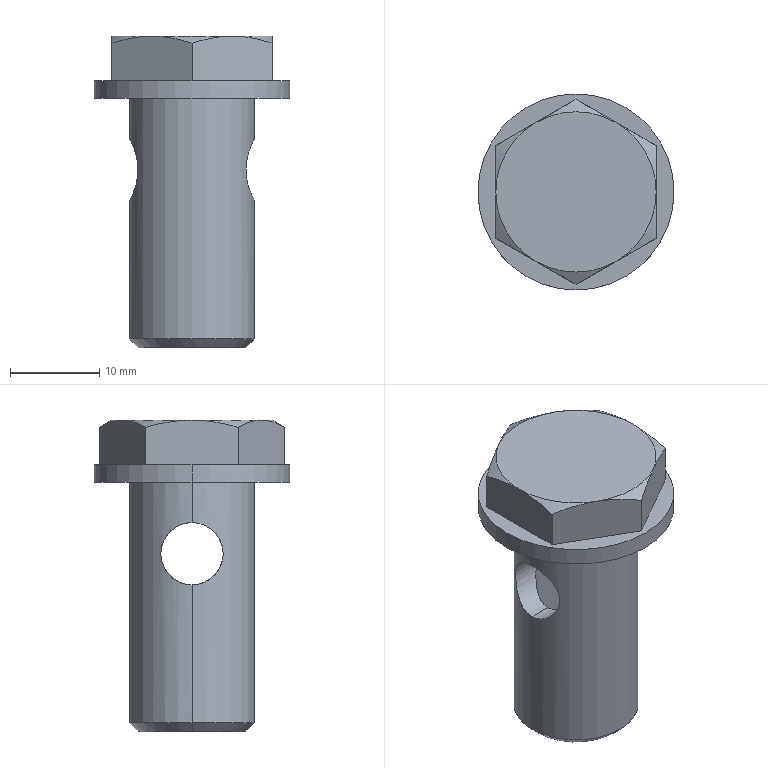Part | SolidWorks | features BaseBody 1 | 1 solid | 32 faces | box 22 x 22 x 35 mm | volume 4530 mm3 | cone 12 | cylinder 10 | plane 10 | commonest cylinder face diameters 7 x4 9 x2 14 x2 22 x2
STEP:
#1=CARTESIAN_POINT('',(49.5,110.5,41.));
#2=VERTEX_POINT('',#1);
#3=CARTESIAN_POINT('',(61.5,110.5,41.));
#4=VERTEX_POINT('',#3);
#5=CARTESIAN_POINT('',(55.5,110.5,41.));
#6=DIRECTION('',(0.,0.,-1.));
#7=DIRECTION('',(-1.,0.,0.));
#8=AXIS2_PLACEMENT_3D('',#5,#6,#7);
#9=CIRCLE('',#8,6.);
#10=EDGE_CURVE('',#2,#4,#9,.T.);
#11=ORIENTED_EDGE('',*,*,#10,.F.);
#12=CARTESIAN_POINT('',(48.5,110.5,42.));
#13=VERTEX_POINT('',#12);
#14=CARTESIAN_POINT('',(49.5,110.5,41.));
#15=DIRECTION('',(-0.7071,0.,0.7071));
#16=VECTOR('',#15,1000.);
#17=LINE('',#14,#16);
#18=EDGE_CURVE('',#2,#13,#17,.T.);
#19=ORIENTED_EDGE('',*,*,#18,.T.);
#20=CARTESIAN_POINT('',(62.5,110.5,42.));
#21=VERTEX_POINT('',#20);
#22=CARTESIAN_POINT('',(55.5,110.5,42.));
#23=DIRECTION('',(0.,0.,1.));
#24=DIRECTION('',(-1.,0.,0.));
#25=AXIS2_PLACEMENT_3D('',#22,#23,#24);
#26=CIRCLE('',#25,7.);
#27=EDGE_CURVE('',#21,#13,#26,.T.);
#28=ORIENTED_EDGE('',*,*,#27,.F.);
#29=CARTESIAN_POINT('',(61.5,110.5,41.));
#30=DIRECTION('',(0.7071,0.,0.7071));
#31=VECTOR('',#30,1000.);
#32=LINE('',#29,#31);
#33=EDGE_CURVE('',#4,#21,#32,.T.);
#34=ORIENTED_EDGE('',*,*,#33,.F.);
#35=EDGE_LOOP('',(#11,#19,#28,#34));
#36=FACE_OUTER_BOUND('',#35,.T.);
#37=CARTESIAN_POINT('',(55.5,110.5,41.));
#38=DIRECTION('',(0.,0.,1.));
#39=DIRECTION('',(1.,0.,0.));
#40=AXIS2_PLACEMENT_3D('',#37,#38,#39);
#41=CONICAL_SURFACE('',#40,6.,0.7854);
#42=ADVANCED_FACE('',(#36),#41,.T.);
#43=CARTESIAN_POINT('',(60.,110.5,41.5));
#44=VERTEX_POINT('',#43);
#45=CARTESIAN_POINT('',(51.,110.5,41.5));
#46=VERTEX_POINT('',#45);
#47=CARTESIAN_POINT('',(55.5,110.5,41.5));
#48=DIRECTION('',(0.,0.,-1.));
#49=DIRECTION('',(-1.,0.,0.));
#50=AXIS2_PLACEMENT_3D('',#47,#48,#49);
#51=CIRCLE('',#50,4.5);
#52=EDGE_CURVE('',#44,#46,#51,.T.);
#53=ORIENTED_EDGE('',*,*,#52,.F.);
#54=CARTESIAN_POINT('',(60.5,110.5,41.));
#55=VERTEX_POINT('',#54);
#56=CARTESIAN_POINT('',(60.,110.5,41.5));
#57=DIRECTION('',(0.7071,0.,-0.7071));
#58=VECTOR('',#57,1000.);
#59=LINE('',#56,#58);
#60=EDGE_CURVE('',#44,#55,#59,.T.);
#61=ORIENTED_EDGE('',*,*,#60,.T.);
#62=CARTESIAN_POINT('',(50.5,110.5,41.));
#63=VERTEX_POINT('',#62);
#64=CARTESIAN_POINT('',(55.5,110.5,41.));
#65=DIRECTION('',(0.,0.,1.));
#66=DIRECTION('',(-1.,0.,0.));
#67=AXIS2_PLACEMENT_3D('',#64,#65,#66);
#68=CIRCLE('',#67,5.);
#69=EDGE_CURVE('',#63,#55,#68,.T.);
#70=ORIENTED_EDGE('',*,*,#69,.F.);
#71=CARTESIAN_POINT('',(51.,110.5,41.5));
#72=DIRECTION('',(-0.7071,0.,-0.7071));
#73=VECTOR('',#72,1000.);
#74=LINE('',#71,#73);
#75=EDGE_CURVE('',#46,#63,#74,.T.);
#76=ORIENTED_EDGE('',*,*,#75,.F.);
#77=EDGE_LOOP('',(#53,#61,#70,#76));
#78=FACE_OUTER_BOUND('',#77,.T.);
#79=CARTESIAN_POINT('',(55.5,110.5,41.5));
#80=DIRECTION('',(0.,0.,-1.));
#81=DIRECTION('',(-1.,0.,0.));
#82=AXIS2_PLACEMENT_3D('',#79,#80,#81);
#83=CONICAL_SURFACE('',#82,4.5,0.7854);
#84=ADVANCED_FACE('',(#78),#83,.F.);
#85=CARTESIAN_POINT('',(51.,110.5,57.5));
#86=VERTEX_POINT('',#85);
#87=CARTESIAN_POINT('',(51.,110.5,64.5));
#88=VERTEX_POINT('',#87);
#89=CARTESIAN_POINT('',(51.,110.5,57.5));
#90=CARTESIAN_POINT('',(51.,110.379,57.5));
#91=CARTESIAN_POINT('',(51.005,110.257,57.506));
#92=CARTESIAN_POINT('',(51.024,110.018,57.531));
#93=CARTESIAN_POINT('',(51.039,109.9,57.55));
#94=CARTESIAN_POINT('',(51.095,109.551,57.623));
#95=CARTESIAN_POINT('',(51.151,109.323,57.696));
#96=CARTESIAN_POINT('',(51.289,108.899,57.879));
#97=CARTESIAN_POINT('',(51.371,108.698,57.991));
#98=CARTESIAN_POINT('',(51.553,108.329,58.246));
#99=CARTESIAN_POINT('',(51.651,108.161,58.388));
#100=CARTESIAN_POINT('',(51.856,107.853,58.699));
#101=CARTESIAN_POINT('',(51.962,107.714,58.87));
#102=CARTESIAN_POINT('',(52.167,107.472,59.231));
#103=CARTESIAN_POINT('',(52.267,107.368,59.423));
#104=CARTESIAN_POINT('',(52.447,107.192,59.836));
#105=CARTESIAN_POINT('',(52.527,107.122,60.056));
#106=CARTESIAN_POINT('',(52.639,107.026,60.516));
#107=CARTESIAN_POINT('',(52.672,107.,60.759));
#108=CARTESIAN_POINT('',(52.672,107.,61.239));
#109=CARTESIAN_POINT('',(52.639,107.025,61.483));
#110=CARTESIAN_POINT('',(52.527,107.121,61.943));
#111=CARTESIAN_POINT('',(52.447,107.192,62.165));
#112=CARTESIAN_POINT('',(52.267,107.367,62.577));
#113=CARTESIAN_POINT('',(52.167,107.472,62.769));
#114=CARTESIAN_POINT('',(51.961,107.715,63.132));
#115=CARTESIAN_POINT('',(51.855,107.855,63.302));
#116=CARTESIAN_POINT('',(51.651,108.161,63.613));
#117=CARTESIAN_POINT('',(51.553,108.329,63.754));
#118=CARTESIAN_POINT('',(51.371,108.698,64.009));
#119=CARTESIAN_POINT('',(51.289,108.899,64.121));
#120=CARTESIAN_POINT('',(51.151,109.322,64.304));
#121=CARTESIAN_POINT('',(51.095,109.55,64.377));
#122=CARTESIAN_POINT('',(51.02,110.017,64.475));
#123=CARTESIAN_POINT('',(51.,110.256,64.5));
#124=CARTESIAN_POINT('',(51.,110.5,64.5));
#125=B_SPLINE_CURVE_WITH_KNOTS('',3,(#89,#90,#91,#92,#93,#94,#95,#96,#97,#98,#99,#100,#101,#102,#103,#104,#105,#106,#107,#108,#109,#110,#111,#112,#113,#114,#115,#116,#117,#118,#119,#120,#121,#122,#123,#124),.UNSPECIFIED.,.F.,.F.,(4,2,2,2,2,2,2,2,2,2,2,2,2,2,2,2,2,4),(0.01153,0.01188,0.01224,0.01296,0.01368,0.0144,0.01512,0.01584,0.01656,0.01727,0.01799,0.01871,0.01943,0.02015,0.02087,0.02159,0.02231,0.02302),.UNSPECIFIED.);
#126=EDGE_CURVE('',#86,#88,#125,.T.);
#127=ORIENTED_EDGE('',*,*,#126,.F.);
#128=CARTESIAN_POINT('',(48.5,110.5,57.5));
#129=VERTEX_POINT('',#128);
#130=CARTESIAN_POINT('',(66.5,110.5,57.5));
#131=DIRECTION('',(-1.,0.,0.));
#132=VECTOR('',#131,1000.);
#133=LINE('',#130,#132);
#134=EDGE_CURVE('',#86,#129,#133,.T.);
#135=ORIENTED_EDGE('',*,*,#134,.T.);
#136=CARTESIAN_POINT('',(48.5,110.5,64.5));
#137=VERTEX_POINT('',#136);
#138=CARTESIAN_POINT('',(48.5,110.5,64.5));
#139=CARTESIAN_POINT('',(48.5,110.264,64.5));
#140=CARTESIAN_POINT('',(48.512,110.034,64.476));
#141=CARTESIAN_POINT('',(48.557,109.581,64.385));
#142=CARTESIAN_POINT('',(48.591,109.356,64.316));
#143=CARTESIAN_POINT('',(48.674,108.933,64.138));
#144=CARTESIAN_POINT('',(48.724,108.734,64.03));
#145=CARTESIAN_POINT('',(48.834,108.356,63.776));
#146=CARTESIAN_POINT('',(48.893,108.181,63.631));
#147=CARTESIAN_POINT('',(49.013,107.864,63.313));
#148=CARTESIAN_POINT('',(49.074,107.72,63.138));
#149=CARTESIAN_POINT('',(49.19,107.467,62.761));
#150=CARTESIAN_POINT('',(49.243,107.36,62.563));
#151=CARTESIAN_POINT('',(49.334,107.184,62.143));
#152=CARTESIAN_POINT('',(49.373,107.115,61.919));
#153=CARTESIAN_POINT('',(49.424,107.023,61.466));
#154=CARTESIAN_POINT('',(49.438,107.,61.236));
#155=CARTESIAN_POINT('',(49.438,107.,60.77));
#156=CARTESIAN_POINT('',(49.424,107.023,60.534));
#157=CARTESIAN_POINT('',(49.373,107.115,60.081));
#158=CARTESIAN_POINT('',(49.335,107.183,59.859));
#159=CARTESIAN_POINT('',(49.243,107.361,59.436));
#160=CARTESIAN_POINT('',(49.189,107.468,59.236));
#161=CARTESIAN_POINT('',(49.074,107.721,58.86));
#162=CARTESIAN_POINT('',(49.012,107.866,58.684));
#163=CARTESIAN_POINT('',(48.892,108.184,58.367));
#164=CARTESIAN_POINT('',(48.833,108.357,58.223));
#165=CARTESIAN_POINT('',(48.723,108.736,57.968));
#166=CARTESIAN_POINT('',(48.673,108.937,57.86));
#167=CARTESIAN_POINT('',(48.591,109.357,57.684));
#168=CARTESIAN_POINT('',(48.557,109.58,57.615));
#169=CARTESIAN_POINT('',(48.512,110.037,57.523));
#170=CARTESIAN_POINT('',(48.5,110.268,57.5));
#171=CARTESIAN_POINT('',(48.5,110.5,57.5));
#172=B_SPLINE_CURVE_WITH_KNOTS('',3,(#138,#139,#140,#141,#142,#143,#144,#145,#146,#147,#148,#149,#150,#151,#152,#153,#154,#155,#156,#157,#158,#159,#160,#161,#162,#163,#164,#165,#166,#167,#168,#169,#170,#171),.UNSPECIFIED.,.F.,.F.,(4,2,2,2,2,2,2,2,2,2,2,2,2,2,2,2,4),(0.,0.0006958,0.001392,0.002088,0.002783,0.003479,0.004175,0.004871,0.005567,0.006263,0.006958,0.007654,0.00835,0.009046,0.009742,0.01044,0.01113),.UNSPECIFIED.);
#173=EDGE_CURVE('',#137,#129,#172,.T.);
#174=ORIENTED_EDGE('',*,*,#173,.F.);
#175=CARTESIAN_POINT('',(66.5,110.5,64.5));
#176=DIRECTION('',(-1.,0.,0.));
#177=VECTOR('',#176,1000.);
#178=LINE('',#175,#177);
#179=EDGE_CURVE('',#88,#137,#178,.T.);
#180=ORIENTED_EDGE('',*,*,#179,.F.);
#181=EDGE_LOOP('',(#127,#135,#174,#180));
#182=FACE_OUTER_BOUND('',#181,.T.);
#183=CARTESIAN_POINT('',(66.5,110.5,61.));
#184=DIRECTION('',(-1.,0.,0.));
#185=DIRECTION('',(0.,0.,1.));
#186=AXIS2_PLACEMENT_3D('',#183,#184,#185);
#187=CYLINDRICAL_SURFACE('',#186,3.5);
#188=ADVANCED_FACE('',(#182),#187,.F.);
#189=CARTESIAN_POINT('',(62.5,110.5,57.5));
#190=VERTEX_POINT('',#189);
#191=CARTESIAN_POINT('',(62.5,110.5,64.5));
#192=VERTEX_POINT('',#191);
#193=CARTESIAN_POINT('',(62.5,110.5,57.5));
#194=CARTESIAN_POINT('',(62.5,110.264,57.5));
#195=CARTESIAN_POINT('',(62.488,110.034,57.524));
#196=CARTESIAN_POINT('',(62.443,109.581,57.615));
#197=CARTESIAN_POINT('',(62.409,109.356,57.684));
#198=CARTESIAN_POINT('',(62.326,108.933,57.862));
#199=CARTESIAN_POINT('',(62.276,108.734,57.97));
#200=CARTESIAN_POINT('',(62.166,108.356,58.224));
#201=CARTESIAN_POINT('',(62.107,108.181,58.369));
#202=CARTESIAN_POINT('',(61.987,107.864,58.687));
#203=CARTESIAN_POINT('',(61.926,107.72,58.862));
#204=CARTESIAN_POINT('',(61.81,107.467,59.239));
#205=CARTESIAN_POINT('',(61.757,107.36,59.437));
#206=CARTESIAN_POINT('',(61.666,107.184,59.857));
#207=CARTESIAN_POINT('',(61.627,107.115,60.081));
#208=CARTESIAN_POINT('',(61.576,107.023,60.534));
#209=CARTESIAN_POINT('',(61.562,107.,60.764));
#210=CARTESIAN_POINT('',(61.562,107.,61.23));
#211=CARTESIAN_POINT('',(61.576,107.023,61.466));
#212=CARTESIAN_POINT('',(61.627,107.115,61.919));
#213=CARTESIAN_POINT('',(61.665,107.183,62.141));
#214=CARTESIAN_POINT('',(61.757,107.361,62.564));
#215=CARTESIAN_POINT('',(61.811,107.468,62.764));
#216=CARTESIAN_POINT('',(61.926,107.721,63.14));
#217=CARTESIAN_POINT('',(61.988,107.866,63.316));
#218=CARTESIAN_POINT('',(62.108,108.184,63.633));
#219=CARTESIAN_POINT('',(62.167,108.357,63.777));
#220=CARTESIAN_POINT('',(62.277,108.736,64.032));
#221=CARTESIAN_POINT('',(62.327,108.937,64.14));
#222=CARTESIAN_POINT('',(62.409,109.357,64.316));
#223=CARTESIAN_POINT('',(62.443,109.58,64.385));
#224=CARTESIAN_POINT('',(62.488,110.037,64.477));
#225=CARTESIAN_POINT('',(62.5,110.268,64.5));
#226=CARTESIAN_POINT('',(62.5,110.5,64.5));
#227=B_SPLINE_CURVE_WITH_KNOTS('',3,(#193,#194,#195,#196,#197,#198,#199,#200,#201,#202,#203,#204,#205,#206,#207,#208,#209,#210,#211,#212,#213,#214,#215,#216,#217,#218,#219,#220,#221,#222,#223,#224,#225,#226),.UNSPECIFIED.,.F.,.F.,(4,2,2,2,2,2,2,2,2,2,2,2,2,2,2,2,4),(0.,0.0006958,0.001392,0.002088,0.002783,0.003479,0.004175,0.004871,0.005567,0.006263,0.006958,0.007654,0.00835,0.009046,0.009742,0.01044,0.01113),.UNSPECIFIED.);
#228=EDGE_CURVE('',#190,#192,#227,.T.);
#229=ORIENTED_EDGE('',*,*,#228,.F.);
#230=CARTESIAN_POINT('',(60.,110.5,57.5));
#231=VERTEX_POINT('',#230);
#232=CARTESIAN_POINT('',(66.5,110.5,57.5));
#233=DIRECTION('',(-1.,0.,0.));
#234=VECTOR('',#233,1000.);
#235=LINE('',#232,#234);
#236=EDGE_CURVE('',#190,#231,#235,.T.);
#237=ORIENTED_EDGE('',*,*,#236,.T.);
#238=CARTESIAN_POINT('',(60.,110.5,64.5));
#239=VERTEX_POINT('',#238);
#240=CARTESIAN_POINT('',(60.,110.5,64.5));
#241=CARTESIAN_POINT('',(60.,110.256,64.5));
#242=CARTESIAN_POINT('',(59.98,110.018,64.475));
#243=CARTESIAN_POINT('',(59.905,109.552,64.378));
#244=CARTESIAN_POINT('',(59.849,109.324,64.304));
#245=CARTESIAN_POINT('',(59.712,108.9,64.121));
#246=CARTESIAN_POINT('',(59.629,108.699,64.01));
#247=CARTESIAN_POINT('',(59.447,108.33,63.755));
#248=CARTESIAN_POINT('',(59.349,108.161,63.613));
#249=CARTESIAN_POINT('',(59.144,107.854,63.301));
#250=CARTESIAN_POINT('',(59.038,107.715,63.131));
#251=CARTESIAN_POINT('',(58.833,107.472,62.769));
#252=CARTESIAN_POINT('',(58.733,107.368,62.578));
#253=CARTESIAN_POINT('',(58.553,107.192,62.164));
#254=CARTESIAN_POINT('',(58.473,107.121,61.944));
#255=CARTESIAN_POINT('',(58.361,107.026,61.484));
#256=CARTESIAN_POINT('',(58.328,107.,61.24));
#257=CARTESIAN_POINT('',(58.328,107.,60.76));
#258=CARTESIAN_POINT('',(58.361,107.026,60.516));
#259=CARTESIAN_POINT('',(58.474,107.122,60.055));
#260=CARTESIAN_POINT('',(58.554,107.192,59.834));
#261=CARTESIAN_POINT('',(58.734,107.368,59.422));
#262=CARTESIAN_POINT('',(58.833,107.473,59.23));
#263=CARTESIAN_POINT('',(59.04,107.717,58.867));
#264=CARTESIAN_POINT('',(59.146,107.856,58.696));
#265=CARTESIAN_POINT('',(59.35,108.162,58.386));
#266=CARTESIAN_POINT('',(59.448,108.33,58.244));
#267=CARTESIAN_POINT('',(59.63,108.701,57.989));
#268=CARTESIAN_POINT('',(59.712,108.901,57.878));
#269=CARTESIAN_POINT('',(59.85,109.325,57.695));
#270=CARTESIAN_POINT('',(59.906,109.553,57.622));
#271=CARTESIAN_POINT('',(59.981,110.02,57.525));
#272=CARTESIAN_POINT('',(60.,110.257,57.5));
#273=CARTESIAN_POINT('',(60.,110.5,57.5));
#274=B_SPLINE_CURVE_WITH_KNOTS('',3,(#240,#241,#242,#243,#244,#245,#246,#247,#248,#249,#250,#251,#252,#253,#254,#255,#256,#257,#258,#259,#260,#261,#262,#263,#264,#265,#266,#267,#268,#269,#270,#271,#272,#273),.UNSPECIFIED.,.F.,.F.,(4,2,2,2,2,2,2,2,2,2,2,2,2,2,2,2,4),(0.,0.0007203,0.001441,0.002161,0.002881,0.003602,0.004322,0.005042,0.005763,0.006483,0.007203,0.007923,0.008644,0.009364,0.01008,0.0108,0.01153),.UNSPECIFIED.);
#275=EDGE_CURVE('',#239,#231,#274,.T.);
#276=ORIENTED_EDGE('',*,*,#275,.F.);
#277=CARTESIAN_POINT('',(66.5,110.5,64.5));
#278=DIRECTION('',(-1.,0.,0.));
#279=VECTOR('',#278,1000.);
#280=LINE('',#277,#279);
#281=EDGE_CURVE('',#192,#239,#280,.T.);
#282=ORIENTED_EDGE('',*,*,#281,.F.);
#283=EDGE_LOOP('',(#229,#237,#276,#282));
#284=FACE_OUTER_BOUND('',#283,.T.);
#285=CARTESIAN_POINT('',(66.5,110.5,61.));
#286=DIRECTION('',(-1.,0.,0.));
#287=DIRECTION('',(0.,0.,1.));
#288=AXIS2_PLACEMENT_3D('',#285,#286,#287);
#289=CYLINDRICAL_SURFACE('',#288,3.5);
#290=ADVANCED_FACE('',(#284),#289,.F.);
#291=CARTESIAN_POINT('',(55.5,110.5,69.598));
#292=VERTEX_POINT('',#291);
#293=CARTESIAN_POINT('',(51.,110.5,67.));
#294=VERTEX_POINT('',#293);
#295=CARTESIAN_POINT('',(51.,110.5,67.));
#296=DIRECTION('',(-0.866,0.,-0.5));
#297=VECTOR('',#296,1000.);
#298=LINE('',#295,#297);
#299=EDGE_CURVE('',#292,#294,#298,.T.);
#300=ORIENTED_EDGE('',*,*,#299,.F.);
#301=CARTESIAN_POINT('',(60.,110.5,67.));
#302=VERTEX_POINT('',#301);
#303=CARTESIAN_POINT('',(60.,110.5,67.));
#304=DIRECTION('',(0.866,0.,-0.5));
#305=VECTOR('',#304,1000.);
#306=LINE('',#303,#305);
#307=EDGE_CURVE('',#292,#302,#306,.T.);
#308=ORIENTED_EDGE('',*,*,#307,.T.);
#309=CARTESIAN_POINT('',(55.5,110.5,67.));
#310=DIRECTION('',(0.,0.,-1.));
#311=DIRECTION('',(-1.,0.,0.));
#312=AXIS2_PLACEMENT_3D('',#309,#310,#311);
#313=CIRCLE('',#312,4.5);
#314=EDGE_CURVE('',#302,#294,#313,.T.);
#315=ORIENTED_EDGE('',*,*,#314,.T.);
#316=EDGE_LOOP('',(#300,#308,#315));
#317=FACE_OUTER_BOUND('',#316,.T.);
#318=CARTESIAN_POINT('',(55.5,110.5,67.));
#319=DIRECTION('',(0.,0.,-1.));
#320=DIRECTION('',(-1.,0.,0.));
#321=AXIS2_PLACEMENT_3D('',#318,#319,#320);
#322=CONICAL_SURFACE('',#321,4.5,1.047);
#323=ADVANCED_FACE('',(#317),#322,.F.);
#324=ORIENTED_EDGE('',*,*,#314,.F.);
#325=CARTESIAN_POINT('',(60.,110.5,67.));
#326=DIRECTION('',(0.,0.,-1.));
#327=VECTOR('',#326,1000.);
#328=LINE('',#325,#327);
#329=EDGE_CURVE('',#302,#239,#328,.T.);
#330=ORIENTED_EDGE('',*,*,#329,.T.);
#331=ORIENTED_EDGE('',*,*,#275,.T.);
#332=CARTESIAN_POINT('',(60.,110.5,67.));
#333=DIRECTION('',(0.,0.,-1.));
#334=VECTOR('',#333,1000.);
#335=LINE('',#332,#334);
#336=EDGE_CURVE('',#231,#44,#335,.T.);
#337=ORIENTED_EDGE('',*,*,#336,.T.);
#338=ORIENTED_EDGE('',*,*,#52,.T.);
#339=CARTESIAN_POINT('',(51.,110.5,67.));
#340=DIRECTION('',(0.,0.,-1.));
#341=VECTOR('',#340,1000.);
#342=LINE('',#339,#341);
#343=EDGE_CURVE('',#86,#46,#342,.T.);
#344=ORIENTED_EDGE('',*,*,#343,.F.);
#345=ORIENTED_EDGE('',*,*,#126,.T.);
#346=CARTESIAN_POINT('',(51.,110.5,67.));
#347=DIRECTION('',(0.,0.,-1.));
#348=VECTOR('',#347,1000.);
#349=LINE('',#346,#348);
#350=EDGE_CURVE('',#294,#88,#349,.T.);
#351=ORIENTED_EDGE('',*,*,#350,.F.);
#352=EDGE_LOOP('',(#324,#330,#331,#337,#338,#344,#345,#351));
#353=FACE_OUTER_BOUND('',#352,.T.);
#354=CARTESIAN_POINT('',(55.5,110.5,67.));
#355=DIRECTION('',(0.,0.,-1.));
#356=DIRECTION('',(-1.,0.,0.));
#357=AXIS2_PLACEMENT_3D('',#354,#355,#356);
#358=CYLINDRICAL_SURFACE('',#357,4.5);
#359=ADVANCED_FACE('',(#353),#358,.F.);
#360=ORIENTED_EDGE('',*,*,#27,.T.);
#361=CARTESIAN_POINT('',(48.5,110.5,41.));
#362=DIRECTION('',(0.,0.,1.));
#363=VECTOR('',#362,1000.);
#364=LINE('',#361,#363);
#365=EDGE_CURVE('',#13,#129,#364,.T.);
#366=ORIENTED_EDGE('',*,*,#365,.T.);
#367=CARTESIAN_POINT('',(48.5,110.5,57.5));
#368=CARTESIAN_POINT('',(48.5,110.732,57.5));
#369=CARTESIAN_POINT('',(48.512,110.968,57.524));
#370=CARTESIAN_POINT('',(48.557,111.422,57.616));
#371=CARTESIAN_POINT('',(48.59,111.642,57.683));
#372=CARTESIAN_POINT('',(48.674,112.068,57.862));
#373=CARTESIAN_POINT('',(48.724,112.268,57.971));
#374=CARTESIAN_POINT('',(48.833,112.643,58.224));
#375=CARTESIAN_POINT('',(48.893,112.82,58.369));
#376=CARTESIAN_POINT('',(49.014,113.137,58.688));
#377=CARTESIAN_POINT('',(49.074,113.279,58.861));
#378=CARTESIAN_POINT('',(49.189,113.531,59.236));
#379=CARTESIAN_POINT('',(49.243,113.641,59.439));
#380=CARTESIAN_POINT('',(49.334,113.816,59.857));
#381=CARTESIAN_POINT('',(49.372,113.884,60.075));
#382=CARTESIAN_POINT('',(49.424,113.976,60.532));
#383=CARTESIAN_POINT('',(49.438,114.,60.765));
#384=CARTESIAN_POINT('',(49.438,114.,61.228));
#385=CARTESIAN_POINT('',(49.424,113.977,61.462));
#386=CARTESIAN_POINT('',(49.373,113.885,61.918));
#387=CARTESIAN_POINT('',(49.336,113.818,62.137));
#388=CARTESIAN_POINT('',(49.198,113.553,62.772));
#389=CARTESIAN_POINT('',(49.074,113.296,63.153));
#390=CARTESIAN_POINT('',(48.893,112.818,63.632));
#391=CARTESIAN_POINT('',(48.834,112.644,63.775));
#392=CARTESIAN_POINT('',(48.725,112.27,64.028));
#393=CARTESIAN_POINT('',(48.674,112.066,64.138));
#394=CARTESIAN_POINT('',(48.591,111.645,64.315));
#395=CARTESIAN_POINT('',(48.558,111.426,64.383));
#396=CARTESIAN_POINT('',(48.512,110.971,64.476));
#397=CARTESIAN_POINT('',(48.5,110.735,64.5));
#398=CARTESIAN_POINT('',(48.5,110.5,64.5));
#399=B_SPLINE_CURVE_WITH_KNOTS('',3,(#367,#368,#369,#370,#371,#372,#373,#374,#375,#376,#377,#378,#379,#380,#381,#382,#383,#384,#385,#386,#387,#388,#389,#390,#391,#392,#393,#394,#395,#396,#397,#398),.UNSPECIFIED.,.F.,.F.,(4,2,2,2,2,2,2,2,2,2,2,2,2,2,2,4),(0.01113,0.01183,0.01252,0.01322,0.01391,0.01461,0.0153,0.016,0.01669,0.01739,0.01808,0.01947,0.02016,0.02086,0.02155,0.02225),.UNSPECIFIED.);
#400=EDGE_CURVE('',#129,#137,#399,.T.);
#401=ORIENTED_EDGE('',*,*,#400,.T.);
#402=CARTESIAN_POINT('',(48.5,110.5,69.));
#403=VERTEX_POINT('',#402);
#404=CARTESIAN_POINT('',(48.5,110.5,41.));
#405=DIRECTION('',(0.,0.,1.));
#406=VECTOR('',#405,1000.);
#407=LINE('',#404,#406);
#408=EDGE_CURVE('',#137,#403,#407,.T.);
#409=ORIENTED_EDGE('',*,*,#408,.T.);
#410=CARTESIAN_POINT('',(62.5,110.5,69.));
#411=VERTEX_POINT('',#410);
#412=CARTESIAN_POINT('',(55.5,110.5,69.));
#413=DIRECTION('',(0.,0.,-1.));
#414=DIRECTION('',(-1.,0.,0.));
#415=AXIS2_PLACEMENT_3D('',#412,#413,#414);
#416=CIRCLE('',#415,7.);
#417=EDGE_CURVE('',#403,#411,#416,.T.);
#418=ORIENTED_EDGE('',*,*,#417,.T.);
#419=CARTESIAN_POINT('',(62.5,110.5,41.));
#420=DIRECTION('',(0.,0.,1.));
#421=VECTOR('',#420,1000.);
#422=LINE('',#419,#421);
#423=EDGE_CURVE('',#192,#411,#422,.T.);
#424=ORIENTED_EDGE('',*,*,#423,.F.);
#425=CARTESIAN_POINT('',(62.5,110.5,64.5));
#426=CARTESIAN_POINT('',(62.5,110.732,64.5));
#427=CARTESIAN_POINT('',(62.488,110.968,64.476));
#428=CARTESIAN_POINT('',(62.443,111.422,64.384));
#429=CARTESIAN_POINT('',(62.41,111.642,64.317));
#430=CARTESIAN_POINT('',(62.326,112.068,64.138));
#431=CARTESIAN_POINT('',(62.276,112.268,64.029));
#432=CARTESIAN_POINT('',(62.167,112.643,63.776));
#433=CARTESIAN_POINT('',(62.107,112.82,63.631));
#434=CARTESIAN_POINT('',(61.986,113.137,63.312));
#435=CARTESIAN_POINT('',(61.926,113.279,63.139));
#436=CARTESIAN_POINT('',(61.811,113.531,62.764));
#437=CARTESIAN_POINT('',(61.757,113.641,62.561));
#438=CARTESIAN_POINT('',(61.666,113.816,62.143));
#439=CARTESIAN_POINT('',(61.628,113.884,61.925));
#440=CARTESIAN_POINT('',(61.576,113.976,61.468));
#441=CARTESIAN_POINT('',(61.562,114.,61.235));
#442=CARTESIAN_POINT('',(61.562,114.,60.772));
#443=CARTESIAN_POINT('',(61.576,113.977,60.538));
#444=CARTESIAN_POINT('',(61.627,113.885,60.082));
#445=CARTESIAN_POINT('',(61.664,113.818,59.863));
#446=CARTESIAN_POINT('',(61.802,113.553,59.228));
#447=CARTESIAN_POINT('',(61.926,113.296,58.847));
#448=CARTESIAN_POINT('',(62.107,112.818,58.368));
#449=CARTESIAN_POINT('',(62.166,112.644,58.225));
#450=CARTESIAN_POINT('',(62.275,112.27,57.972));
#451=CARTESIAN_POINT('',(62.326,112.066,57.862));
#452=CARTESIAN_POINT('',(62.409,111.645,57.685));
#453=CARTESIAN_POINT('',(62.442,111.426,57.617));
#454=CARTESIAN_POINT('',(62.488,110.971,57.524));
#455=CARTESIAN_POINT('',(62.5,110.735,57.5));
#456=CARTESIAN_POINT('',(62.5,110.5,57.5));
#457=B_SPLINE_CURVE_WITH_KNOTS('',3,(#425,#426,#427,#428,#429,#430,#431,#432,#433,#434,#435,#436,#437,#438,#439,#440,#441,#442,#443,#444,#445,#446,#447,#448,#449,#450,#451,#452,#453,#454,#455,#456),.UNSPECIFIED.,.F.,.F.,(4,2,2,2,2,2,2,2,2,2,2,2,2,2,2,4),(0.01113,0.01183,0.01252,0.01322,0.01391,0.01461,0.0153,0.016,0.01669,0.01739,0.01808,0.01947,0.02016,0.02086,0.02155,0.02225),.UNSPECIFIED.);
#458=EDGE_CURVE('',#192,#190,#457,.T.);
#459=ORIENTED_EDGE('',*,*,#458,.T.);
#460=CARTESIAN_POINT('',(62.5,110.5,41.));
#461=DIRECTION('',(0.,0.,1.));
#462=VECTOR('',#461,1000.);
#463=LINE('',#460,#462);
#464=EDGE_CURVE('',#21,#190,#463,.T.);
#465=ORIENTED_EDGE('',*,*,#464,.F.);
#466=EDGE_LOOP('',(#360,#366,#401,#409,#418,#424,#459,#465));
#467=FACE_OUTER_BOUND('',#466,.T.);
#468=CARTESIAN_POINT('',(55.5,110.5,41.));
#469=DIRECTION('',(0.,0.,1.));
#470=DIRECTION('',(1.,0.,0.));
#471=AXIS2_PLACEMENT_3D('',#468,#469,#470);
#472=CYLINDRICAL_SURFACE('',#471,7.);
#473=ADVANCED_FACE('',(#467),#472,.T.);
#474=CARTESIAN_POINT('',(44.5,110.5,69.));
#475=VERTEX_POINT('',#474);
#476=CARTESIAN_POINT('',(66.5,110.5,69.));
#477=VERTEX_POINT('',#476);
#478=CARTESIAN_POINT('',(55.5,110.5,69.));
#479=DIRECTION('',(0.,0.,-1.));
#480=DIRECTION('',(-1.,0.,0.));
#481=AXIS2_PLACEMENT_3D('',#478,#479,#480);
#482=CIRCLE('',#481,11.);
#483=EDGE_CURVE('',#475,#477,#482,.T.);
#484=ORIENTED_EDGE('',*,*,#483,.F.);
#485=CARTESIAN_POINT('',(44.5,110.5,71.));
#486=VERTEX_POINT('',#485);
#487=CARTESIAN_POINT('',(44.5,110.5,69.));
#488=DIRECTION('',(0.,0.,1.));
#489=VECTOR('',#488,1000.);
#490=LINE('',#487,#489);
#491=EDGE_CURVE('',#475,#486,#490,.T.);
#492=ORIENTED_EDGE('',*,*,#491,.T.);
#493=CARTESIAN_POINT('',(66.5,110.5,71.));
#494=VERTEX_POINT('',#493);
#495=CARTESIAN_POINT('',(55.5,110.5,71.));
#496=DIRECTION('',(0.,0.,-1.));
#497=DIRECTION('',(-1.,0.,0.));
#498=AXIS2_PLACEMENT_3D('',#495,#496,#497);
#499=CIRCLE('',#498,11.);
#500=EDGE_CURVE('',#486,#494,#499,.T.);
#501=ORIENTED_EDGE('',*,*,#500,.T.);
#502=CARTESIAN_POINT('',(66.5,110.5,69.));
#503=DIRECTION('',(0.,0.,1.));
#504=VECTOR('',#503,1000.);
#505=LINE('',#502,#504);
#506=EDGE_CURVE('',#477,#494,#505,.T.);
#507=ORIENTED_EDGE('',*,*,#506,.F.);
#508=EDGE_LOOP('',(#484,#492,#501,#507));
#509=FACE_OUTER_BOUND('',#508,.T.);
#510=CARTESIAN_POINT('',(55.5,110.5,69.));
#511=DIRECTION('',(0.,0.,1.));
#512=DIRECTION('',(1.,0.,0.));
#513=AXIS2_PLACEMENT_3D('',#510,#511,#512);
#514=CYLINDRICAL_SURFACE('',#513,11.);
#515=ADVANCED_FACE('',(#509),#514,.T.);
#516=CARTESIAN_POINT('',(55.5,120.892,75.196));
#517=VERTEX_POINT('',#516);
#518=CARTESIAN_POINT('',(51.,118.294,76.));
#519=VERTEX_POINT('',#518);
#520=CARTESIAN_POINT('',(55.5,120.892,75.196));
#521=CARTESIAN_POINT('',(54.764,120.467,75.442));
#522=CARTESIAN_POINT('',(54.022,120.039,75.644));
#523=CARTESIAN_POINT('',(52.524,119.174,75.923));
#524=CARTESIAN_POINT('',(51.767,118.737,76.));
#525=CARTESIAN_POINT('',(51.,118.294,76.));
#526=B_SPLINE_CURVE_WITH_KNOTS('',3,(#520,#521,#522,#523,#524,#525),.UNSPECIFIED.,.F.,.F.,(4,2,4),(0.000000238,0.002629,0.005258),.UNSPECIFIED.);
#527=EDGE_CURVE('',#517,#519,#526,.T.);
#528=ORIENTED_EDGE('',*,*,#527,.F.);
#529=CARTESIAN_POINT('',(55.5,120.892,71.));
#530=VERTEX_POINT('',#529);
#531=CARTESIAN_POINT('',(55.5,120.892,71.));
#532=DIRECTION('',(0.,0.,1.));
#533=VECTOR('',#532,1000.);
#534=LINE('',#531,#533);
#535=EDGE_CURVE('',#530,#517,#534,.T.);
#536=ORIENTED_EDGE('',*,*,#535,.F.);
#537=CARTESIAN_POINT('',(46.5,115.696,71.));
#538=VERTEX_POINT('',#537);
#539=CARTESIAN_POINT('',(46.5,115.696,71.));
#540=DIRECTION('',(0.866,0.5,0.));
#541=VECTOR('',#540,1000.);
#542=LINE('',#539,#541);
#543=EDGE_CURVE('',#538,#530,#542,.T.);
#544=ORIENTED_EDGE('',*,*,#543,.F.);
#545=CARTESIAN_POINT('',(46.5,115.696,75.196));
#546=VERTEX_POINT('',#545);
#547=CARTESIAN_POINT('',(46.5,115.696,71.));
#548=DIRECTION('',(0.,0.,1.));
#549=VECTOR('',#548,1000.);
#550=LINE('',#547,#549);
#551=EDGE_CURVE('',#538,#546,#550,.T.);
#552=ORIENTED_EDGE('',*,*,#551,.T.);
#553=CARTESIAN_POINT('',(51.,118.294,76.));
#554=CARTESIAN_POINT('',(50.618,118.074,76.));
#555=CARTESIAN_POINT('',(50.234,117.852,75.981));
#556=CARTESIAN_POINT('',(49.476,117.414,75.907));
#557=CARTESIAN_POINT('',(49.099,117.197,75.853));
#558=CARTESIAN_POINT('',(47.975,116.548,75.643));
#559=CARTESIAN_POINT('',(47.234,116.12,75.441));
#560=CARTESIAN_POINT('',(46.5,115.696,75.196));
#561=B_SPLINE_CURVE_WITH_KNOTS('',3,(#553,#554,#555,#556,#557,#558,#559,#560),.UNSPECIFIED.,.F.,.F.,(4,2,2,4),(0.005258,0.006567,0.007877,0.0105),.UNSPECIFIED.);
#562=EDGE_CURVE('',#519,#546,#561,.T.);
#563=ORIENTED_EDGE('',*,*,#562,.F.);
#564=EDGE_LOOP('',(#528,#536,#544,#552,#563));
#565=FACE_OUTER_BOUND('',#564,.T.);
#566=CARTESIAN_POINT('',(46.5,115.696,71.));
#567=DIRECTION('',(0.5,-0.866,0.));
#568=DIRECTION('',(-0.866,-0.5,0.));
#569=AXIS2_PLACEMENT_3D('',#566,#567,#568);
#570=PLANE('',#569);
#571=ADVANCED_FACE('',(#565),#570,.F.);
#572=CARTESIAN_POINT('',(64.5,115.696,75.196));
#573=VERTEX_POINT('',#572);
#574=CARTESIAN_POINT('',(60.,118.294,76.));
#575=VERTEX_POINT('',#574);
#576=CARTESIAN_POINT('',(64.5,115.696,75.196));
#577=CARTESIAN_POINT('',(63.764,116.121,75.442));
#578=CARTESIAN_POINT('',(63.022,116.549,75.644));
#579=CARTESIAN_POINT('',(61.524,117.414,75.923));
#580=CARTESIAN_POINT('',(60.767,117.852,76.));
#581=CARTESIAN_POINT('',(60.,118.294,76.));
#582=B_SPLINE_CURVE_WITH_KNOTS('',3,(#576,#577,#578,#579,#580,#581),.UNSPECIFIED.,.F.,.F.,(4,2,4),(0.000000238,0.002629,0.005258),.UNSPECIFIED.);
#583=EDGE_CURVE('',#573,#575,#582,.T.);
#584=ORIENTED_EDGE('',*,*,#583,.F.);
#585=CARTESIAN_POINT('',(64.5,115.696,71.));
#586=VERTEX_POINT('',#585);
#587=CARTESIAN_POINT('',(64.5,115.696,71.));
#588=DIRECTION('',(0.,0.,1.));
#589=VECTOR('',#588,1000.);
#590=LINE('',#587,#589);
#591=EDGE_CURVE('',#586,#573,#590,.T.);
#592=ORIENTED_EDGE('',*,*,#591,.F.);
#593=CARTESIAN_POINT('',(55.5,120.892,71.));
#594=DIRECTION('',(0.866,-0.5,0.));
#595=VECTOR('',#594,1000.);
#596=LINE('',#593,#595);
#597=EDGE_CURVE('',#530,#586,#596,.T.);
#598=ORIENTED_EDGE('',*,*,#597,.F.);
#599=ORIENTED_EDGE('',*,*,#535,.T.);
#600=CARTESIAN_POINT('',(60.,118.294,76.));
#601=CARTESIAN_POINT('',(59.618,118.515,76.));
#602=CARTESIAN_POINT('',(59.234,118.736,75.981));
#603=CARTESIAN_POINT('',(58.476,119.174,75.907));
#604=CARTESIAN_POINT('',(58.099,119.392,75.853));
#605=CARTESIAN_POINT('',(56.975,120.041,75.643));
#606=CARTESIAN_POINT('',(56.234,120.468,75.441));
#607=CARTESIAN_POINT('',(55.5,120.892,75.196));
#608=B_SPLINE_CURVE_WITH_KNOTS('',3,(#600,#601,#602,#603,#604,#605,#606,#607),.UNSPECIFIED.,.F.,.F.,(4,2,2,4),(0.005258,0.006567,0.007877,0.0105),.UNSPECIFIED.);
#609=EDGE_CURVE('',#575,#517,#608,.T.);
#610=ORIENTED_EDGE('',*,*,#609,.F.);
#611=EDGE_LOOP('',(#584,#592,#598,#599,#610));
#612=FACE_OUTER_BOUND('',#611,.T.);
#613=CARTESIAN_POINT('',(55.5,120.892,71.));
#614=DIRECTION('',(-0.5,-0.866,0.));
#615=DIRECTION('',(-0.866,0.5,0.));
#616=AXIS2_PLACEMENT_3D('',#613,#614,#615);
#617=PLANE('',#616);
#618=ADVANCED_FACE('',(#612),#617,.F.);
#619=CARTESIAN_POINT('',(64.5,105.304,75.196));
#620=VERTEX_POINT('',#619);
#621=CARTESIAN_POINT('',(64.5,110.5,76.));
#622=VERTEX_POINT('',#621);
#623=CARTESIAN_POINT('',(64.5,105.304,75.196));
#624=CARTESIAN_POINT('',(64.5,106.15,75.44));
#625=CARTESIAN_POINT('',(64.5,107.015,75.645));
#626=CARTESIAN_POINT('',(64.5,108.749,75.924));
#627=CARTESIAN_POINT('',(64.5,109.621,76.));
#628=CARTESIAN_POINT('',(64.5,110.5,76.));
#629=B_SPLINE_CURVE_WITH_KNOTS('',3,(#623,#624,#625,#626,#627,#628),.UNSPECIFIED.,.F.,.F.,(4,2,4),(0.009533,0.01216,0.01479),.UNSPECIFIED.);
#630=EDGE_CURVE('',#620,#622,#629,.T.);
#631=ORIENTED_EDGE('',*,*,#630,.F.);
#632=CARTESIAN_POINT('',(64.5,105.304,71.));
#633=VERTEX_POINT('',#632);
#634=CARTESIAN_POINT('',(64.5,105.304,71.));
#635=DIRECTION('',(0.,0.,1.));
#636=VECTOR('',#635,1000.);
#637=LINE('',#634,#636);
#638=EDGE_CURVE('',#633,#620,#637,.T.);
#639=ORIENTED_EDGE('',*,*,#638,.F.);
#640=CARTESIAN_POINT('',(64.5,115.696,71.));
#641=DIRECTION('',(0.,-1.,0.));
#642=VECTOR('',#641,1000.);
#643=LINE('',#640,#642);
#644=EDGE_CURVE('',#586,#633,#643,.T.);
#645=ORIENTED_EDGE('',*,*,#644,.F.);
#646=ORIENTED_EDGE('',*,*,#591,.T.);
#647=CARTESIAN_POINT('',(64.5,110.5,76.));
#648=CARTESIAN_POINT('',(64.5,110.94,76.));
#649=CARTESIAN_POINT('',(64.5,111.382,75.981));
#650=CARTESIAN_POINT('',(64.5,112.266,75.907));
#651=CARTESIAN_POINT('',(64.5,112.704,75.852));
#652=CARTESIAN_POINT('',(64.5,114.005,75.641));
#653=CARTESIAN_POINT('',(64.5,114.856,75.439));
#654=CARTESIAN_POINT('',(64.5,115.696,75.196));
#655=B_SPLINE_CURVE_WITH_KNOTS('',3,(#647,#648,#649,#650,#651,#652,#653,#654),.UNSPECIFIED.,.F.,.F.,(4,2,2,4),(0.01479,0.01611,0.01742,0.02006),.UNSPECIFIED.);
#656=EDGE_CURVE('',#622,#573,#655,.T.);
#657=ORIENTED_EDGE('',*,*,#656,.F.);
#658=EDGE_LOOP('',(#631,#639,#645,#646,#657));
#659=FACE_OUTER_BOUND('',#658,.T.);
#660=CARTESIAN_POINT('',(64.5,115.696,71.));
#661=DIRECTION('',(-1.,0.,0.));
#662=DIRECTION('',(0.,0.,1.));
#663=AXIS2_PLACEMENT_3D('',#660,#661,#662);
#664=PLANE('',#663);
#665=ADVANCED_FACE('',(#659),#664,.F.);
#666=CARTESIAN_POINT('',(55.5,100.108,75.196));
#667=VERTEX_POINT('',#666);
#668=CARTESIAN_POINT('',(60.,102.706,76.));
#669=VERTEX_POINT('',#668);
#670=CARTESIAN_POINT('',(55.5,100.108,75.196));
#671=CARTESIAN_POINT('',(56.236,100.533,75.442));
#672=CARTESIAN_POINT('',(56.978,100.961,75.644));
#673=CARTESIAN_POINT('',(58.476,101.826,75.923));
#674=CARTESIAN_POINT('',(59.233,102.263,76.));
#675=CARTESIAN_POINT('',(60.,102.706,76.));
#676=B_SPLINE_CURVE_WITH_KNOTS('',3,(#670,#671,#672,#673,#674,#675),.UNSPECIFIED.,.F.,.F.,(4,2,4),(0.000000238,0.002629,0.005258),.UNSPECIFIED.);
#677=EDGE_CURVE('',#667,#669,#676,.T.);
#678=ORIENTED_EDGE('',*,*,#677,.F.);
#679=CARTESIAN_POINT('',(55.5,100.108,71.));
#680=VERTEX_POINT('',#679);
#681=CARTESIAN_POINT('',(55.5,100.108,71.));
#682=DIRECTION('',(0.,0.,1.));
#683=VECTOR('',#682,1000.);
#684=LINE('',#681,#683);
#685=EDGE_CURVE('',#680,#667,#684,.T.);
#686=ORIENTED_EDGE('',*,*,#685,.F.);
#687=CARTESIAN_POINT('',(64.5,105.304,71.));
#688=DIRECTION('',(-0.866,-0.5,0.));
#689=VECTOR('',#688,1000.);
#690=LINE('',#687,#689);
#691=EDGE_CURVE('',#633,#680,#690,.T.);
#692=ORIENTED_EDGE('',*,*,#691,.F.);
#693=ORIENTED_EDGE('',*,*,#638,.T.);
#694=CARTESIAN_POINT('',(60.,102.706,76.));
#695=CARTESIAN_POINT('',(60.382,102.926,76.));
#696=CARTESIAN_POINT('',(60.766,103.148,75.981));
#697=CARTESIAN_POINT('',(61.524,103.586,75.907));
#698=CARTESIAN_POINT('',(61.901,103.803,75.853));
#699=CARTESIAN_POINT('',(63.025,104.452,75.643));
#700=CARTESIAN_POINT('',(63.766,104.88,75.441));
#701=CARTESIAN_POINT('',(64.5,105.304,75.196));
#702=B_SPLINE_CURVE_WITH_KNOTS('',3,(#694,#695,#696,#697,#698,#699,#700,#701),.UNSPECIFIED.,.F.,.F.,(4,2,2,4),(0.005258,0.006567,0.007877,0.0105),.UNSPECIFIED.);
#703=EDGE_CURVE('',#669,#620,#702,.T.);
#704=ORIENTED_EDGE('',*,*,#703,.F.);
#705=EDGE_LOOP('',(#678,#686,#692,#693,#704));
#706=FACE_OUTER_BOUND('',#705,.T.);
#707=CARTESIAN_POINT('',(64.5,105.304,71.));
#708=DIRECTION('',(-0.5,0.866,0.));
#709=DIRECTION('',(0.866,0.5,0.));
#710=AXIS2_PLACEMENT_3D('',#707,#708,#709);
#711=PLANE('',#710);
#712=ADVANCED_FACE('',(#706),#711,.F.);
#713=CARTESIAN_POINT('',(46.5,105.304,75.196));
#714=VERTEX_POINT('',#713);
#715=CARTESIAN_POINT('',(51.,102.706,76.));
#716=VERTEX_POINT('',#715);
#717=CARTESIAN_POINT('',(46.5,105.304,75.196));
#718=CARTESIAN_POINT('',(47.236,104.879,75.442));
#719=CARTESIAN_POINT('',(47.978,104.451,75.644));
#720=CARTESIAN_POINT('',(49.476,103.586,75.923));
#721=CARTESIAN_POINT('',(50.233,103.148,76.));
#722=CARTESIAN_POINT('',(51.,102.706,76.));
#723=B_SPLINE_CURVE_WITH_KNOTS('',3,(#717,#718,#719,#720,#721,#722),.UNSPECIFIED.,.F.,.F.,(4,2,4),(0.000000238,0.002629,0.005258),.UNSPECIFIED.);
#724=EDGE_CURVE('',#714,#716,#723,.T.);
#725=ORIENTED_EDGE('',*,*,#724,.F.);
#726=CARTESIAN_POINT('',(46.5,105.304,71.));
#727=VERTEX_POINT('',#726);
#728=CARTESIAN_POINT('',(46.5,105.304,71.));
#729=DIRECTION('',(0.,0.,1.));
#730=VECTOR('',#729,1000.);
#731=LINE('',#728,#730);
#732=EDGE_CURVE('',#727,#714,#731,.T.);
#733=ORIENTED_EDGE('',*,*,#732,.F.);
#734=CARTESIAN_POINT('',(55.5,100.108,71.));
#735=DIRECTION('',(-0.866,0.5,0.));
#736=VECTOR('',#735,1000.);
#737=LINE('',#734,#736);
#738=EDGE_CURVE('',#680,#727,#737,.T.);
#739=ORIENTED_EDGE('',*,*,#738,.F.);
#740=ORIENTED_EDGE('',*,*,#685,.T.);
#741=CARTESIAN_POINT('',(51.,102.706,76.));
#742=CARTESIAN_POINT('',(51.382,102.485,76.));
#743=CARTESIAN_POINT('',(51.766,102.264,75.981));
#744=CARTESIAN_POINT('',(52.524,101.826,75.907));
#745=CARTESIAN_POINT('',(52.901,101.608,75.853));
#746=CARTESIAN_POINT('',(54.025,100.959,75.643));
#747=CARTESIAN_POINT('',(54.766,100.532,75.441));
#748=CARTESIAN_POINT('',(55.5,100.108,75.196));
#749=B_SPLINE_CURVE_WITH_KNOTS('',3,(#741,#742,#743,#744,#745,#746,#747,#748),.UNSPECIFIED.,.F.,.F.,(4,2,2,4),(0.005258,0.006567,0.007877,0.0105),.UNSPECIFIED.);
#750=EDGE_CURVE('',#716,#667,#749,.T.);
#751=ORIENTED_EDGE('',*,*,#750,.F.);
#752=EDGE_LOOP('',(#725,#733,#739,#740,#751));
#753=FACE_OUTER_BOUND('',#752,.T.);
#754=CARTESIAN_POINT('',(55.5,100.108,71.));
#755=DIRECTION('',(0.5,0.866,0.));
#756=DIRECTION('',(0.866,-0.5,0.));
#757=AXIS2_PLACEMENT_3D('',#754,#755,#756);
#758=PLANE('',#757);
#759=ADVANCED_FACE('',(#753),#758,.F.);
#760=CARTESIAN_POINT('',(46.5,110.5,76.));
#761=VERTEX_POINT('',#760);
#762=CARTESIAN_POINT('',(46.5,115.696,75.196));
#763=CARTESIAN_POINT('',(46.5,114.856,75.439));
#764=CARTESIAN_POINT('',(46.5,114.005,75.641));
#765=CARTESIAN_POINT('',(46.5,112.704,75.852));
#766=CARTESIAN_POINT('',(46.5,112.266,75.907));
#767=CARTESIAN_POINT('',(46.5,111.382,75.981));
#768=CARTESIAN_POINT('',(46.5,110.94,76.));
#769=CARTESIAN_POINT('',(46.5,110.5,76.));
#770=B_SPLINE_CURVE_WITH_KNOTS('',3,(#762,#763,#764,#765,#766,#767,#768,#769),.UNSPECIFIED.,.F.,.F.,(4,2,2,4),(0.0266,0.02923,0.03055,0.03187),.UNSPECIFIED.);
#771=EDGE_CURVE('',#546,#761,#770,.T.);
#772=ORIENTED_EDGE('',*,*,#771,.F.);
#773=ORIENTED_EDGE('',*,*,#551,.F.);
#774=CARTESIAN_POINT('',(46.5,105.304,71.));
#775=DIRECTION('',(0.,1.,0.));
#776=VECTOR('',#775,1000.);
#777=LINE('',#774,#776);
#778=EDGE_CURVE('',#727,#538,#777,.T.);
#779=ORIENTED_EDGE('',*,*,#778,.F.);
#780=ORIENTED_EDGE('',*,*,#732,.T.);
#781=CARTESIAN_POINT('',(46.5,110.5,76.));
#782=CARTESIAN_POINT('',(46.5,109.621,76.));
#783=CARTESIAN_POINT('',(46.5,108.749,75.924));
#784=CARTESIAN_POINT('',(46.5,107.015,75.645));
#785=CARTESIAN_POINT('',(46.5,106.15,75.44));
#786=CARTESIAN_POINT('',(46.5,105.304,75.196));
#787=B_SPLINE_CURVE_WITH_KNOTS('',3,(#781,#782,#783,#784,#785,#786),.UNSPECIFIED.,.F.,.F.,(4,2,4),(0.03187,0.03449,0.03712),.UNSPECIFIED.);
#788=EDGE_CURVE('',#761,#714,#787,.T.);
#789=ORIENTED_EDGE('',*,*,#788,.F.);
#790=EDGE_LOOP('',(#772,#773,#779,#780,#789));
#791=FACE_OUTER_BOUND('',#790,.T.);
#792=CARTESIAN_POINT('',(46.5,105.304,71.));
#793=DIRECTION('',(1.,0.,0.));
#794=DIRECTION('',(0.,-1.,0.));
#795=AXIS2_PLACEMENT_3D('',#792,#793,#794);
#796=PLANE('',#795);
#797=ADVANCED_FACE('',(#791),#796,.F.);
#798=CARTESIAN_POINT('',(55.5,110.5,69.));
#799=DIRECTION('',(0.,0.,-1.));
#800=DIRECTION('',(-1.,0.,0.));
#801=AXIS2_PLACEMENT_3D('',#798,#799,#800);
#802=CIRCLE('',#801,11.);
#803=EDGE_CURVE('',#477,#475,#802,.T.);
#804=ORIENTED_EDGE('',*,*,#803,.T.);
#805=ORIENTED_EDGE('',*,*,#483,.T.);
#806=EDGE_LOOP('',(#804,#805));
#807=FACE_OUTER_BOUND('',#806,.T.);
#808=CARTESIAN_POINT('',(55.5,110.5,69.));
#809=DIRECTION('',(0.,0.,-1.));
#810=DIRECTION('',(-1.,0.,0.));
#811=AXIS2_PLACEMENT_3D('',#808,#809,#810);
#812=CIRCLE('',#811,7.);
#813=EDGE_CURVE('',#411,#403,#812,.T.);
#814=ORIENTED_EDGE('',*,*,#813,.F.);
#815=ORIENTED_EDGE('',*,*,#417,.F.);
#816=EDGE_LOOP('',(#814,#815));
#817=FACE_BOUND('',#816,.T.);
#818=CARTESIAN_POINT('',(55.5,110.5,69.));
#819=DIRECTION('',(0.,0.,-1.));
#820=DIRECTION('',(-1.,0.,0.));
#821=AXIS2_PLACEMENT_3D('',#818,#819,#820);
#822=PLANE('',#821);
#823=ADVANCED_FACE('',(#807,#817),#822,.T.);
#824=CARTESIAN_POINT('',(55.5,110.5,71.));
#825=DIRECTION('',(0.,0.,-1.));
#826=DIRECTION('',(-1.,0.,0.));
#827=AXIS2_PLACEMENT_3D('',#824,#825,#826);
#828=CIRCLE('',#827,11.);
#829=EDGE_CURVE('',#494,#486,#828,.T.);
#830=ORIENTED_EDGE('',*,*,#829,.F.);
#831=ORIENTED_EDGE('',*,*,#500,.F.);
#832=EDGE_LOOP('',(#830,#831));
#833=FACE_OUTER_BOUND('',#832,.T.);
#834=ORIENTED_EDGE('',*,*,#778,.T.);
#835=ORIENTED_EDGE('',*,*,#543,.T.);
#836=ORIENTED_EDGE('',*,*,#597,.T.);
#837=ORIENTED_EDGE('',*,*,#644,.T.);
#838=ORIENTED_EDGE('',*,*,#691,.T.);
#839=ORIENTED_EDGE('',*,*,#738,.T.);
#840=EDGE_LOOP('',(#834,#835,#836,#837,#838,#839));
#841=FACE_BOUND('',#840,.T.);
#842=CARTESIAN_POINT('',(55.5,110.5,71.));
#843=DIRECTION('',(0.,0.,-1.));
#844=DIRECTION('',(-1.,0.,0.));
#845=AXIS2_PLACEMENT_3D('',#842,#843,#844);
#846=PLANE('',#845);
#847=ADVANCED_FACE('',(#833,#841),#846,.F.);
#848=ORIENTED_EDGE('',*,*,#491,.F.);
#849=ORIENTED_EDGE('',*,*,#803,.F.);
#850=ORIENTED_EDGE('',*,*,#506,.T.);
#851=ORIENTED_EDGE('',*,*,#829,.T.);
#852=EDGE_LOOP('',(#848,#849,#850,#851));
#853=FACE_OUTER_BOUND('',#852,.T.);
#854=CARTESIAN_POINT('',(55.5,110.5,69.));
#855=DIRECTION('',(0.,0.,1.));
#856=DIRECTION('',(1.,0.,0.));
#857=AXIS2_PLACEMENT_3D('',#854,#855,#856);
#858=CYLINDRICAL_SURFACE('',#857,11.);
#859=ADVANCED_FACE('',(#853),#858,.T.);
#860=ORIENTED_EDGE('',*,*,#365,.F.);
#861=CARTESIAN_POINT('',(55.5,110.5,42.));
#862=DIRECTION('',(0.,0.,1.));
#863=DIRECTION('',(-1.,0.,0.));
#864=AXIS2_PLACEMENT_3D('',#861,#862,#863);
#865=CIRCLE('',#864,7.);
#866=EDGE_CURVE('',#13,#21,#865,.T.);
#867=ORIENTED_EDGE('',*,*,#866,.T.);
#868=ORIENTED_EDGE('',*,*,#464,.T.);
#869=ORIENTED_EDGE('',*,*,#228,.T.);
#870=ORIENTED_EDGE('',*,*,#423,.T.);
#871=ORIENTED_EDGE('',*,*,#813,.T.);
#872=ORIENTED_EDGE('',*,*,#408,.F.);
#873=ORIENTED_EDGE('',*,*,#173,.T.);
#874=EDGE_LOOP('',(#860,#867,#868,#869,#870,#871,#872,#873));
#875=FACE_OUTER_BOUND('',#874,.T.);
#876=CARTESIAN_POINT('',(55.5,110.5,41.));
#877=DIRECTION('',(0.,0.,1.));
#878=DIRECTION('',(1.,0.,0.));
#879=AXIS2_PLACEMENT_3D('',#876,#877,#878);
#880=CYLINDRICAL_SURFACE('',#879,7.);
#881=ADVANCED_FACE('',(#875),#880,.T.);
#882=CARTESIAN_POINT('',(55.5,110.5,41.));
#883=DIRECTION('',(0.,0.,-1.));
#884=DIRECTION('',(-1.,0.,0.));
#885=AXIS2_PLACEMENT_3D('',#882,#883,#884);
#886=CIRCLE('',#885,6.);
#887=EDGE_CURVE('',#4,#2,#886,.T.);
#888=ORIENTED_EDGE('',*,*,#887,.T.);
#889=ORIENTED_EDGE('',*,*,#10,.T.);
#890=EDGE_LOOP('',(#888,#889));
#891=FACE_OUTER_BOUND('',#890,.T.);
#892=ORIENTED_EDGE('',*,*,#69,.T.);
#893=CARTESIAN_POINT('',(55.5,110.5,41.));
#894=DIRECTION('',(0.,0.,1.));
#895=DIRECTION('',(-1.,0.,0.));
#896=AXIS2_PLACEMENT_3D('',#893,#894,#895);
#897=CIRCLE('',#896,5.);
#898=EDGE_CURVE('',#55,#63,#897,.T.);
#899=ORIENTED_EDGE('',*,*,#898,.T.);
#900=EDGE_LOOP('',(#892,#899));
#901=FACE_BOUND('',#900,.T.);
#902=CARTESIAN_POINT('',(55.5,110.5,41.));
#903=DIRECTION('',(0.,0.,-1.));
#904=DIRECTION('',(-1.,0.,0.));
#905=AXIS2_PLACEMENT_3D('',#902,#903,#904);
#906=PLANE('',#905);
#907=ADVANCED_FACE('',(#891,#901),#906,.T.);
#908=ORIENTED_EDGE('',*,*,#329,.F.);
#909=CARTESIAN_POINT('',(55.5,110.5,67.));
#910=DIRECTION('',(0.,0.,-1.));
#911=DIRECTION('',(-1.,0.,0.));
#912=AXIS2_PLACEMENT_3D('',#909,#910,#911);
#913=CIRCLE('',#912,4.5);
#914=EDGE_CURVE('',#294,#302,#913,.T.);
#915=ORIENTED_EDGE('',*,*,#914,.F.);
#916=ORIENTED_EDGE('',*,*,#350,.T.);
#917=CARTESIAN_POINT('',(51.,110.5,64.5));
#918=CARTESIAN_POINT('',(51.,110.744,64.5));
#919=CARTESIAN_POINT('',(51.02,110.982,64.475));
#920=CARTESIAN_POINT('',(51.095,111.448,64.378));
#921=CARTESIAN_POINT('',(51.151,111.676,64.304));
#922=CARTESIAN_POINT('',(51.288,112.1,64.121));
#923=CARTESIAN_POINT('',(51.371,112.301,64.01));
#924=CARTESIAN_POINT('',(51.553,112.67,63.755));
#925=CARTESIAN_POINT('',(51.651,112.839,63.613));
#926=CARTESIAN_POINT('',(51.856,113.146,63.301));
#927=CARTESIAN_POINT('',(51.962,113.285,63.131));
#928=CARTESIAN_POINT('',(52.167,113.528,62.769));
#929=CARTESIAN_POINT('',(52.267,113.632,62.578));
#930=CARTESIAN_POINT('',(52.447,113.808,62.164));
#931=CARTESIAN_POINT('',(52.527,113.879,61.944));
#932=CARTESIAN_POINT('',(52.639,113.974,61.484));
#933=CARTESIAN_POINT('',(52.672,114.,61.24));
#934=CARTESIAN_POINT('',(52.672,114.,60.76));
#935=CARTESIAN_POINT('',(52.639,113.974,60.516));
#936=CARTESIAN_POINT('',(52.526,113.878,60.055));
#937=CARTESIAN_POINT('',(52.446,113.808,59.834));
#938=CARTESIAN_POINT('',(52.266,113.632,59.422));
#939=CARTESIAN_POINT('',(52.167,113.527,59.23));
#940=CARTESIAN_POINT('',(51.96,113.283,58.867));
#941=CARTESIAN_POINT('',(51.854,113.144,58.696));
#942=CARTESIAN_POINT('',(51.65,112.838,58.386));
#943=CARTESIAN_POINT('',(51.552,112.67,58.244));
#944=CARTESIAN_POINT('',(51.37,112.299,57.989));
#945=CARTESIAN_POINT('',(51.288,112.099,57.878));
#946=CARTESIAN_POINT('',(51.15,111.675,57.695));
#947=CARTESIAN_POINT('',(51.094,111.447,57.622));
#948=CARTESIAN_POINT('',(51.019,110.98,57.525));
#949=CARTESIAN_POINT('',(51.,110.743,57.5));
#950=CARTESIAN_POINT('',(51.,110.5,57.5));
#951=B_SPLINE_CURVE_WITH_KNOTS('',3,(#917,#918,#919,#920,#921,#922,#923,#924,#925,#926,#927,#928,#929,#930,#931,#932,#933,#934,#935,#936,#937,#938,#939,#940,#941,#942,#943,#944,#945,#946,#947,#948,#949,#950),.UNSPECIFIED.,.F.,.F.,(4,2,2,2,2,2,2,2,2,2,2,2,2,2,2,2,4),(0.,0.0007203,0.001441,0.002161,0.002881,0.003602,0.004322,0.005042,0.005763,0.006483,0.007203,0.007923,0.008644,0.009364,0.01008,0.0108,0.01153),.UNSPECIFIED.);
#952=EDGE_CURVE('',#88,#86,#951,.T.);
#953=ORIENTED_EDGE('',*,*,#952,.T.);
#954=ORIENTED_EDGE('',*,*,#343,.T.);
#955=CARTESIAN_POINT('',(55.5,110.5,41.5));
#956=DIRECTION('',(0.,0.,-1.));
#957=DIRECTION('',(-1.,0.,0.));
#958=AXIS2_PLACEMENT_3D('',#955,#956,#957);
#959=CIRCLE('',#958,4.5);
#960=EDGE_CURVE('',#46,#44,#959,.T.);
#961=ORIENTED_EDGE('',*,*,#960,.T.);
#962=ORIENTED_EDGE('',*,*,#336,.F.);
#963=CARTESIAN_POINT('',(60.,110.5,57.5));
#964=CARTESIAN_POINT('',(60.,110.621,57.5));
#965=CARTESIAN_POINT('',(59.995,110.743,57.506));
#966=CARTESIAN_POINT('',(59.976,110.982,57.531));
#967=CARTESIAN_POINT('',(59.961,111.1,57.55));
#968=CARTESIAN_POINT('',(59.905,111.449,57.623));
#969=CARTESIAN_POINT('',(59.849,111.677,57.696));
#970=CARTESIAN_POINT('',(59.711,112.101,57.879));
#971=CARTESIAN_POINT('',(59.629,112.302,57.991));
#972=CARTESIAN_POINT('',(59.447,112.671,58.246));
#973=CARTESIAN_POINT('',(59.349,112.839,58.388));
#974=CARTESIAN_POINT('',(59.144,113.147,58.699));
#975=CARTESIAN_POINT('',(59.038,113.286,58.87));
#976=CARTESIAN_POINT('',(58.833,113.528,59.231));
#977=CARTESIAN_POINT('',(58.733,113.632,59.423));
#978=CARTESIAN_POINT('',(58.553,113.808,59.836));
#979=CARTESIAN_POINT('',(58.473,113.878,60.056));
#980=CARTESIAN_POINT('',(58.361,113.974,60.516));
#981=CARTESIAN_POINT('',(58.328,114.,60.759));
#982=CARTESIAN_POINT('',(58.328,114.,61.239));
#983=CARTESIAN_POINT('',(58.361,113.975,61.483));
#984=CARTESIAN_POINT('',(58.473,113.879,61.943));
#985=CARTESIAN_POINT('',(58.553,113.808,62.165));
#986=CARTESIAN_POINT('',(58.733,113.633,62.577));
#987=CARTESIAN_POINT('',(58.833,113.528,62.769));
#988=CARTESIAN_POINT('',(59.039,113.285,63.132));
#989=CARTESIAN_POINT('',(59.145,113.145,63.302));
#990=CARTESIAN_POINT('',(59.349,112.839,63.613));
#991=CARTESIAN_POINT('',(59.447,112.671,63.754));
#992=CARTESIAN_POINT('',(59.629,112.302,64.009));
#993=CARTESIAN_POINT('',(59.711,112.101,64.121));
#994=CARTESIAN_POINT('',(59.849,111.678,64.304));
#995=CARTESIAN_POINT('',(59.905,111.45,64.377));
#996=CARTESIAN_POINT('',(59.98,110.983,64.475));
#997=CARTESIAN_POINT('',(60.,110.744,64.5));
#998=CARTESIAN_POINT('',(60.,110.5,64.5));
#999=B_SPLINE_CURVE_WITH_KNOTS('',3,(#963,#964,#965,#966,#967,#968,#969,#970,#971,#972,#973,#974,#975,#976,#977,#978,#979,#980,#981,#982,#983,#984,#985,#986,#987,#988,#989,#990,#991,#992,#993,#994,#995,#996,#997,#998),.UNSPECIFIED.,.F.,.F.,(4,2,2,2,2,2,2,2,2,2,2,2,2,2,2,2,2,4),(0.01153,0.01188,0.01224,0.01296,0.01368,0.0144,0.01512,0.01584,0.01656,0.01727,0.01799,0.01871,0.01943,0.02015,0.02087,0.02159,0.02231,0.02302),.UNSPECIFIED.);
#1000=EDGE_CURVE('',#231,#239,#999,.T.);
#1001=ORIENTED_EDGE('',*,*,#1000,.T.);
#1002=EDGE_LOOP('',(#908,#915,#916,#953,#954,#961,#962,#1001));
#1003=FACE_OUTER_BOUND('',#1002,.T.);
#1004=CARTESIAN_POINT('',(55.5,110.5,67.));
#1005=DIRECTION('',(0.,0.,-1.));
#1006=DIRECTION('',(-1.,0.,0.));
#1007=AXIS2_PLACEMENT_3D('',#1004,#1005,#1006);
#1008=CYLINDRICAL_SURFACE('',#1007,4.5);
#1009=ADVANCED_FACE('',(#1003),#1008,.F.);
#1010=ORIENTED_EDGE('',*,*,#307,.F.);
#1011=ORIENTED_EDGE('',*,*,#299,.T.);
#1012=ORIENTED_EDGE('',*,*,#914,.T.);
#1013=EDGE_LOOP('',(#1010,#1011,#1012));
#1014=FACE_OUTER_BOUND('',#1013,.T.);
#1015=CARTESIAN_POINT('',(55.5,110.5,67.));
#1016=DIRECTION('',(0.,0.,-1.));
#1017=DIRECTION('',(-1.,0.,0.));
#1018=AXIS2_PLACEMENT_3D('',#1015,#1016,#1017);
#1019=CONICAL_SURFACE('',#1018,4.5,1.047);
#1020=ADVANCED_FACE('',(#1014),#1019,.F.);
#1021=ORIENTED_EDGE('',*,*,#236,.F.);
#1022=ORIENTED_EDGE('',*,*,#458,.F.);
#1023=ORIENTED_EDGE('',*,*,#281,.T.);
#1024=ORIENTED_EDGE('',*,*,#1000,.F.);
#1025=EDGE_LOOP('',(#1021,#1022,#1023,#1024));
#1026=FACE_OUTER_BOUND('',#1025,.T.);
#1027=CARTESIAN_POINT('',(66.5,110.5,61.));
#1028=DIRECTION('',(-1.,0.,0.));
#1029=DIRECTION('',(0.,0.,1.));
#1030=AXIS2_PLACEMENT_3D('',#1027,#1028,#1029);
#1031=CYLINDRICAL_SURFACE('',#1030,3.5);
#1032=ADVANCED_FACE('',(#1026),#1031,.F.);
#1033=ORIENTED_EDGE('',*,*,#134,.F.);
#1034=ORIENTED_EDGE('',*,*,#952,.F.);
#1035=ORIENTED_EDGE('',*,*,#179,.T.);
#1036=ORIENTED_EDGE('',*,*,#400,.F.);
#1037=EDGE_LOOP('',(#1033,#1034,#1035,#1036));
#1038=FACE_OUTER_BOUND('',#1037,.T.);
#1039=CARTESIAN_POINT('',(66.5,110.5,61.));
#1040=DIRECTION('',(-1.,0.,0.));
#1041=DIRECTION('',(0.,0.,1.));
#1042=AXIS2_PLACEMENT_3D('',#1039,#1040,#1041);
#1043=CYLINDRICAL_SURFACE('',#1042,3.5);
#1044=ADVANCED_FACE('',(#1038),#1043,.F.);
#1045=ORIENTED_EDGE('',*,*,#60,.F.);
#1046=ORIENTED_EDGE('',*,*,#960,.F.);
#1047=ORIENTED_EDGE('',*,*,#75,.T.);
#1048=ORIENTED_EDGE('',*,*,#898,.F.);
#1049=EDGE_LOOP('',(#1045,#1046,#1047,#1048));
#1050=FACE_OUTER_BOUND('',#1049,.T.);
#1051=CARTESIAN_POINT('',(55.5,110.5,41.5));
#1052=DIRECTION('',(0.,0.,-1.));
#1053=DIRECTION('',(-1.,0.,0.));
#1054=AXIS2_PLACEMENT_3D('',#1051,#1052,#1053);
#1055=CONICAL_SURFACE('',#1054,4.5,0.7854);
#1056=ADVANCED_FACE('',(#1050),#1055,.F.);
#1057=ORIENTED_EDGE('',*,*,#724,.T.);
#1058=CARTESIAN_POINT('',(55.5,110.5,76.));
#1059=DIRECTION('',(0.,0.,-1.));
#1060=DIRECTION('',(-1.,0.,0.));
#1061=AXIS2_PLACEMENT_3D('',#1058,#1059,#1060);
#1062=CIRCLE('',#1061,9.);
#1063=EDGE_CURVE('',#716,#761,#1062,.T.);
#1064=ORIENTED_EDGE('',*,*,#1063,.T.);
#1065=ORIENTED_EDGE('',*,*,#788,.T.);
#1066=EDGE_LOOP('',(#1057,#1064,#1065));
#1067=FACE_OUTER_BOUND('',#1066,.T.);
#1068=CARTESIAN_POINT('',(55.5,110.5,76.));
#1069=DIRECTION('',(0.,0.,-1.));
#1070=DIRECTION('',(1.,0.,0.));
#1071=AXIS2_PLACEMENT_3D('',#1068,#1069,#1070);
#1072=CONICAL_SURFACE('',#1071,9.,1.047);
#1073=ADVANCED_FACE('',(#1067),#1072,.T.);
#1074=ORIENTED_EDGE('',*,*,#677,.T.);
#1075=CARTESIAN_POINT('',(55.5,110.5,76.));
#1076=DIRECTION('',(0.,0.,-1.));
#1077=DIRECTION('',(-1.,0.,0.));
#1078=AXIS2_PLACEMENT_3D('',#1075,#1076,#1077);
#1079=CIRCLE('',#1078,9.);
#1080=EDGE_CURVE('',#669,#716,#1079,.T.);
#1081=ORIENTED_EDGE('',*,*,#1080,.T.);
#1082=ORIENTED_EDGE('',*,*,#750,.T.);
#1083=EDGE_LOOP('',(#1074,#1081,#1082));
#1084=FACE_OUTER_BOUND('',#1083,.T.);
#1085=CARTESIAN_POINT('',(55.5,110.5,76.));
#1086=DIRECTION('',(0.,0.,-1.));
#1087=DIRECTION('',(1.,0.,0.));
#1088=AXIS2_PLACEMENT_3D('',#1085,#1086,#1087);
#1089=CONICAL_SURFACE('',#1088,9.,1.047);
#1090=ADVANCED_FACE('',(#1084),#1089,.T.);
#1091=ORIENTED_EDGE('',*,*,#630,.T.);
#1092=CARTESIAN_POINT('',(55.5,110.5,76.));
#1093=DIRECTION('',(0.,0.,-1.));
#1094=DIRECTION('',(-1.,0.,0.));
#1095=AXIS2_PLACEMENT_3D('',#1092,#1093,#1094);
#1096=CIRCLE('',#1095,9.);
#1097=EDGE_CURVE('',#622,#669,#1096,.T.);
#1098=ORIENTED_EDGE('',*,*,#1097,.T.);
#1099=ORIENTED_EDGE('',*,*,#703,.T.);
#1100=EDGE_LOOP('',(#1091,#1098,#1099));
#1101=FACE_OUTER_BOUND('',#1100,.T.);
#1102=CARTESIAN_POINT('',(55.5,110.5,76.));
#1103=DIRECTION('',(0.,0.,-1.));
#1104=DIRECTION('',(1.,0.,0.));
#1105=AXIS2_PLACEMENT_3D('',#1102,#1103,#1104);
#1106=CONICAL_SURFACE('',#1105,9.,1.047);
#1107=ADVANCED_FACE('',(#1101),#1106,.T.);
#1108=ORIENTED_EDGE('',*,*,#656,.T.);
#1109=ORIENTED_EDGE('',*,*,#583,.T.);
#1110=CARTESIAN_POINT('',(55.5,110.5,76.));
#1111=DIRECTION('',(0.,0.,1.));
#1112=DIRECTION('',(1.,0.,0.));
#1113=AXIS2_PLACEMENT_3D('',#1110,#1111,#1112);
#1114=CIRCLE('',#1113,9.);
#1115=EDGE_CURVE('',#622,#575,#1114,.T.);
#1116=ORIENTED_EDGE('',*,*,#1115,.F.);
#1117=EDGE_LOOP('',(#1108,#1109,#1116));
#1118=FACE_OUTER_BOUND('',#1117,.T.);
#1119=CARTESIAN_POINT('',(55.5,110.5,76.));
#1120=DIRECTION('',(0.,0.,-1.));
#1121=DIRECTION('',(1.,0.,0.));
#1122=AXIS2_PLACEMENT_3D('',#1119,#1120,#1121);
#1123=CONICAL_SURFACE('',#1122,9.,1.047);
#1124=ADVANCED_FACE('',(#1118),#1123,.T.);
#1125=ORIENTED_EDGE('',*,*,#609,.T.);
#1126=ORIENTED_EDGE('',*,*,#527,.T.);
#1127=CARTESIAN_POINT('',(55.5,110.5,76.));
#1128=DIRECTION('',(0.,0.,-1.));
#1129=DIRECTION('',(-1.,0.,0.));
#1130=AXIS2_PLACEMENT_3D('',#1127,#1128,#1129);
#1131=CIRCLE('',#1130,9.);
#1132=EDGE_CURVE('',#519,#575,#1131,.T.);
#1133=ORIENTED_EDGE('',*,*,#1132,.T.);
#1134=EDGE_LOOP('',(#1125,#1126,#1133));
#1135=FACE_OUTER_BOUND('',#1134,.T.);
#1136=CARTESIAN_POINT('',(55.5,110.5,76.));
#1137=DIRECTION('',(0.,0.,-1.));
#1138=DIRECTION('',(1.,0.,0.));
#1139=AXIS2_PLACEMENT_3D('',#1136,#1137,#1138);
#1140=CONICAL_SURFACE('',#1139,9.,1.047);
#1141=ADVANCED_FACE('',(#1135),#1140,.T.);
#1142=ORIENTED_EDGE('',*,*,#562,.T.);
#1143=ORIENTED_EDGE('',*,*,#771,.T.);
#1144=CARTESIAN_POINT('',(55.5,110.5,76.));
#1145=DIRECTION('',(0.,0.,-1.));
#1146=DIRECTION('',(-1.,0.,0.));
#1147=AXIS2_PLACEMENT_3D('',#1144,#1145,#1146);
#1148=CIRCLE('',#1147,9.);
#1149=EDGE_CURVE('',#761,#519,#1148,.T.);
#1150=ORIENTED_EDGE('',*,*,#1149,.T.);
#1151=EDGE_LOOP('',(#1142,#1143,#1150));
#1152=FACE_OUTER_BOUND('',#1151,.T.);
#1153=CARTESIAN_POINT('',(55.5,110.5,76.));
#1154=DIRECTION('',(0.,0.,-1.));
#1155=DIRECTION('',(1.,0.,0.));
#1156=AXIS2_PLACEMENT_3D('',#1153,#1154,#1155);
#1157=CONICAL_SURFACE('',#1156,9.,1.047);
#1158=ADVANCED_FACE('',(#1152),#1157,.T.);
#1159=ORIENTED_EDGE('',*,*,#1149,.F.);
#1160=ORIENTED_EDGE('',*,*,#1063,.F.);
#1161=ORIENTED_EDGE('',*,*,#1080,.F.);
#1162=ORIENTED_EDGE('',*,*,#1097,.F.);
#1163=ORIENTED_EDGE('',*,*,#1115,.T.);
#1164=ORIENTED_EDGE('',*,*,#1132,.F.);
#1165=EDGE_LOOP('',(#1159,#1160,#1161,#1162,#1163,#1164));
#1166=FACE_OUTER_BOUND('',#1165,.T.);
#1167=CARTESIAN_POINT('',(55.5,120.892,76.));
#1168=DIRECTION('',(0.,0.,-1.));
#1169=DIRECTION('',(-1.,0.,0.));
#1170=AXIS2_PLACEMENT_3D('',#1167,#1168,#1169);
#1171=PLANE('',#1170);
#1172=ADVANCED_FACE('',(#1166),#1171,.F.);
#1173=ORIENTED_EDGE('',*,*,#18,.F.);
#1174=ORIENTED_EDGE('',*,*,#887,.F.);
#1175=ORIENTED_EDGE('',*,*,#33,.T.);
#1176=ORIENTED_EDGE('',*,*,#866,.F.);
#1177=EDGE_LOOP('',(#1173,#1174,#1175,#1176));
#1178=FACE_OUTER_BOUND('',#1177,.T.);
#1179=CARTESIAN_POINT('',(55.5,110.5,41.));
#1180=DIRECTION('',(0.,0.,1.));
#1181=DIRECTION('',(1.,0.,0.));
#1182=AXIS2_PLACEMENT_3D('',#1179,#1180,#1181);
#1183=CONICAL_SURFACE('',#1182,6.,0.7854);
#1184=ADVANCED_FACE('',(#1178),#1183,.T.);
#1185=CLOSED_SHELL('',(#42,#84,#188,#290,#323,#359,#473,#515,#571,#618,#665,#712,#759,#797,#823,#847,#859,#881,#907,#1009,#1020,#1032,#1044,#1056,#1073,#1090,#1107,#1124,#1141,#1158,#1172,#1184));
#1186=MANIFOLD_SOLID_BREP('',#1185);
#1187=CARTESIAN_POINT('',(0.,0.,0.));
#1188=DIRECTION('',(0.,0.,1.));
#1189=DIRECTION('',(1.,0.,0.));
#1190=AXIS2_PLACEMENT_3D('',#1187,#1188,#1189);
#1191=(LENGTH_UNIT()NAMED_UNIT(*)SI_UNIT(.MILLI.,.METRE.));
#1192=UNCERTAINTY_MEASURE_WITH_UNIT(LENGTH_MEASURE(0.00001),#1191,'','');
#1193=(NAMED_UNIT(*)PLANE_ANGLE_UNIT()SI_UNIT($,.RADIAN.));
#1194=(NAMED_UNIT(*)SI_UNIT($,.STERADIAN.)SOLID_ANGLE_UNIT());
#1195=(GEOMETRIC_REPRESENTATION_CONTEXT(3)GLOBAL_UNCERTAINTY_ASSIGNED_CONTEXT((#1192))GLOBAL_UNIT_ASSIGNED_CONTEXT((#1191,#1193,#1194))REPRESENTATION_CONTEXT('',''));
#1196=ADVANCED_BREP_SHAPE_REPRESENTATION('',(#1186,#1190),#1195);